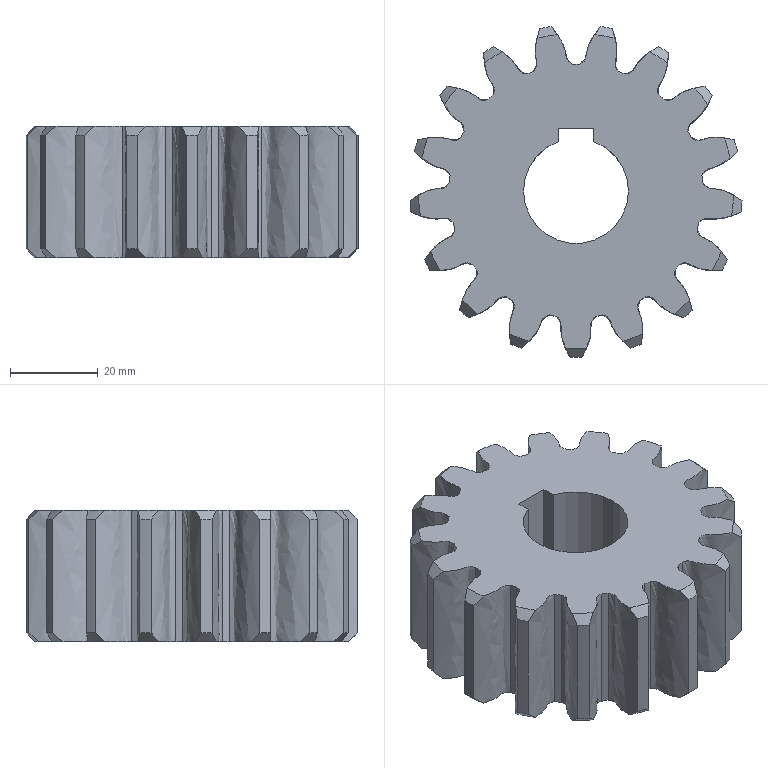Part | SolidWorks | features ICE 5, Chamfer 3, CirPattern 1, Extrusion 1, RefAxis 1 | 1 solid | 110 faces | box 75.876 x 75.576 x 30 mm | volume 92447 mm3 | cylinder 37 | cone 34 | spline 34 | plane 5 | commonest cylinder face diameters 58 x17 76 x17 24 x3